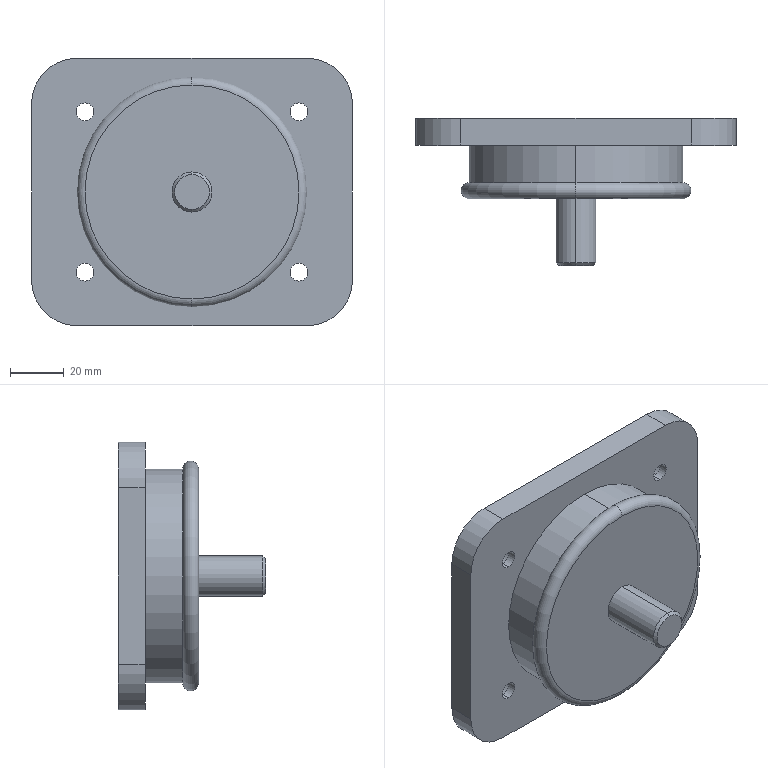Part | SolidWorks | features ICE 3, Chamfer 1, Extrusion 1, HoleWzd 1, Revolution 1 | 1 solid | 58 faces | box 120 x 55 x 100 mm | volume 210377 mm3 | cylinder 29 | cone 14 | plane 13 | torus 2 | commonest cylinder face diameters 6.6 x8 11 x8 90 x5 34 x4 15 x2 80 x2